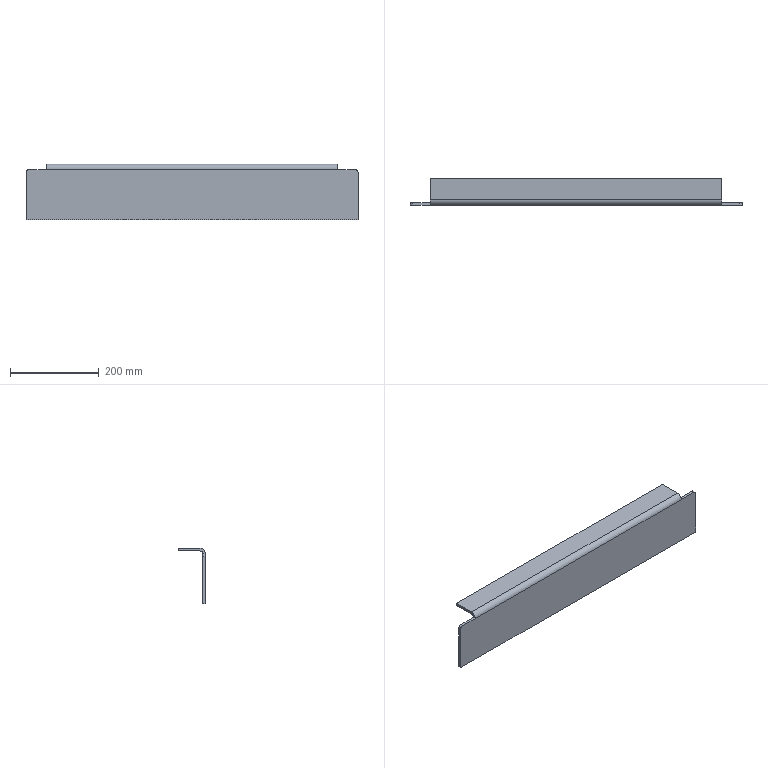Part | NX | features solid 2 | 1 solid | 16 faces | box 750 x 60 x 125 mm | volume 753725 mm3 | plane 12 | cylinder 4 | commonest cylinder face diameters 12 x3 24 x1
STEP:
#1=CARTESIAN_POINT('',(-345.,50.,-225.));
#2=VERTEX_POINT('',#1);
#3=CARTESIAN_POINT('',(-351.,50.,-219.));
#4=VERTEX_POINT('',#3);
#5=CARTESIAN_POINT('',(-351.,50.,-225.));
#6=DIRECTION('',(0.,-1.,0.));
#7=DIRECTION('',(-1.,0.,0.));
#8=AXIS2_PLACEMENT_3D('',#5,#6,#7);
#9=CIRCLE('',#8,6.);
#10=EDGE_CURVE('',#2,#4,#9,.T.);
#11=ORIENTED_EDGE('',*,*,#10,.F.);
#12=CARTESIAN_POINT('',(-345.,56.,-225.));
#13=VERTEX_POINT('',#12);
#14=CARTESIAN_POINT('',(-345.,48.,-225.));
#15=DIRECTION('',(0.,-1.,0.));
#16=VECTOR('',#15,1000.);
#17=LINE('',#14,#16);
#18=EDGE_CURVE('',#13,#2,#17,.T.);
#19=ORIENTED_EDGE('',*,*,#18,.F.);
#20=CARTESIAN_POINT('',(-351.,56.,-219.));
#21=VERTEX_POINT('',#20);
#22=CARTESIAN_POINT('',(-351.,56.,-225.));
#23=DIRECTION('',(0.,1.,0.));
#24=DIRECTION('',(-1.,0.,0.));
#25=AXIS2_PLACEMENT_3D('',#22,#23,#24);
#26=CIRCLE('',#25,6.);
#27=EDGE_CURVE('',#21,#13,#26,.T.);
#28=ORIENTED_EDGE('',*,*,#27,.F.);
#29=CARTESIAN_POINT('',(-351.,56.,-219.));
#30=DIRECTION('',(0.,1.,0.));
#31=VECTOR('',#30,1000.);
#32=LINE('',#29,#31);
#33=EDGE_CURVE('',#4,#21,#32,.T.);
#34=ORIENTED_EDGE('',*,*,#33,.F.);
#35=EDGE_LOOP('',(#11,#19,#28,#34));
#36=FACE_BOUND('',#35,.T.);
#37=CARTESIAN_POINT('',(-351.,56.,-225.));
#38=DIRECTION('',(0.,1.,0.));
#39=DIRECTION('',(-1.,0.,0.));
#40=AXIS2_PLACEMENT_3D('',#37,#38,#39);
#41=CYLINDRICAL_SURFACE('',#40,6.);
#42=ADVANCED_FACE('',(#36),#41,.T.);
#43=CARTESIAN_POINT('',(-1089.,50.,-219.));
#44=VERTEX_POINT('',#43);
#45=CARTESIAN_POINT('',(-1095.,50.,-225.));
#46=VERTEX_POINT('',#45);
#47=CARTESIAN_POINT('',(-1089.,50.,-225.));
#48=DIRECTION('',(0.,-1.,0.));
#49=DIRECTION('',(-1.,0.,0.));
#50=AXIS2_PLACEMENT_3D('',#47,#48,#49);
#51=CIRCLE('',#50,6.);
#52=EDGE_CURVE('',#44,#46,#51,.T.);
#53=ORIENTED_EDGE('',*,*,#52,.F.);
#54=CARTESIAN_POINT('',(-1089.,56.,-219.));
#55=VERTEX_POINT('',#54);
#56=CARTESIAN_POINT('',(-1089.,56.,-219.));
#57=DIRECTION('',(0.,-1.,0.));
#58=VECTOR('',#57,1000.);
#59=LINE('',#56,#58);
#60=EDGE_CURVE('',#55,#44,#59,.T.);
#61=ORIENTED_EDGE('',*,*,#60,.F.);
#62=CARTESIAN_POINT('',(-1095.,56.,-225.));
#63=VERTEX_POINT('',#62);
#64=CARTESIAN_POINT('',(-1089.,56.,-225.));
#65=DIRECTION('',(0.,1.,0.));
#66=DIRECTION('',(-1.,0.,0.));
#67=AXIS2_PLACEMENT_3D('',#64,#65,#66);
#68=CIRCLE('',#67,6.);
#69=EDGE_CURVE('',#63,#55,#68,.T.);
#70=ORIENTED_EDGE('',*,*,#69,.F.);
#71=CARTESIAN_POINT('',(-1095.,48.,-225.));
#72=DIRECTION('',(0.,1.,0.));
#73=VECTOR('',#72,1000.);
#74=LINE('',#71,#73);
#75=EDGE_CURVE('',#46,#63,#74,.T.);
#76=ORIENTED_EDGE('',*,*,#75,.F.);
#77=EDGE_LOOP('',(#53,#61,#70,#76));
#78=FACE_BOUND('',#77,.T.);
#79=CARTESIAN_POINT('',(-1089.,48.,-225.));
#80=DIRECTION('',(0.,1.,0.));
#81=DIRECTION('',(-1.,0.,0.));
#82=AXIS2_PLACEMENT_3D('',#79,#80,#81);
#83=CYLINDRICAL_SURFACE('',#82,6.);
#84=ADVANCED_FACE('',(#78),#83,.T.);
#85=CARTESIAN_POINT('',(-391.,62.,-213.));
#86=VERTEX_POINT('',#85);
#87=CARTESIAN_POINT('',(-391.,56.,-219.));
#88=VERTEX_POINT('',#87);
#89=CARTESIAN_POINT('',(-391.,62.,-219.));
#90=DIRECTION('',(1.,0.,0.));
#91=DIRECTION('',(0.,-1.,0.));
#92=AXIS2_PLACEMENT_3D('',#89,#90,#91);
#93=CIRCLE('',#92,6.);
#94=EDGE_CURVE('',#86,#88,#93,.T.);
#95=ORIENTED_EDGE('',*,*,#94,.T.);
#96=CARTESIAN_POINT('',(-1049.,56.,-219.));
#97=VERTEX_POINT('',#96);
#98=CARTESIAN_POINT('',(-1095.,56.,-219.));
#99=DIRECTION('',(-1.,0.,0.));
#100=VECTOR('',#99,1000.);
#101=LINE('',#98,#100);
#102=EDGE_CURVE('',#88,#97,#101,.T.);
#103=ORIENTED_EDGE('',*,*,#102,.T.);
#104=CARTESIAN_POINT('',(-1049.,62.,-213.));
#105=VERTEX_POINT('',#104);
#106=CARTESIAN_POINT('',(-1049.,62.,-219.));
#107=DIRECTION('',(-1.,0.,0.));
#108=DIRECTION('',(0.,-1.,0.));
#109=AXIS2_PLACEMENT_3D('',#106,#107,#108);
#110=CIRCLE('',#109,6.);
#111=EDGE_CURVE('',#97,#105,#110,.T.);
#112=ORIENTED_EDGE('',*,*,#111,.T.);
#113=CARTESIAN_POINT('',(-1049.,62.,-213.));
#114=DIRECTION('',(1.,0.,0.));
#115=VECTOR('',#114,1000.);
#116=LINE('',#113,#115);
#117=EDGE_CURVE('',#105,#86,#116,.T.);
#118=ORIENTED_EDGE('',*,*,#117,.T.);
#119=EDGE_LOOP('',(#95,#103,#112,#118));
#120=FACE_BOUND('',#119,.T.);
#121=CARTESIAN_POINT('',(-1095.,62.,-219.));
#122=DIRECTION('',(1.,0.,0.));
#123=DIRECTION('',(0.,1.,0.));
#124=AXIS2_PLACEMENT_3D('',#121,#122,#123);
#125=CYLINDRICAL_SURFACE('',#124,6.);
#126=ADVANCED_FACE('',(#120),#125,.F.);
#127=CARTESIAN_POINT('',(-391.,62.,-207.));
#128=VERTEX_POINT('',#127);
#129=CARTESIAN_POINT('',(-391.,50.,-219.));
#130=VERTEX_POINT('',#129);
#131=CARTESIAN_POINT('',(-391.,62.,-219.));
#132=DIRECTION('',(1.,0.,0.));
#133=DIRECTION('',(0.,1.,0.));
#134=AXIS2_PLACEMENT_3D('',#131,#132,#133);
#135=CIRCLE('',#134,12.);
#136=EDGE_CURVE('',#128,#130,#135,.T.);
#137=ORIENTED_EDGE('',*,*,#136,.F.);
#138=CARTESIAN_POINT('',(-1049.,62.,-207.));
#139=VERTEX_POINT('',#138);
#140=CARTESIAN_POINT('',(-1049.,62.,-207.));
#141=DIRECTION('',(1.,0.,0.));
#142=VECTOR('',#141,1000.);
#143=LINE('',#140,#142);
#144=EDGE_CURVE('',#139,#128,#143,.T.);
#145=ORIENTED_EDGE('',*,*,#144,.F.);
#146=CARTESIAN_POINT('',(-1049.,50.,-219.));
#147=VERTEX_POINT('',#146);
#148=CARTESIAN_POINT('',(-1049.,62.,-219.));
#149=DIRECTION('',(-1.,0.,0.));
#150=DIRECTION('',(0.,1.,0.));
#151=AXIS2_PLACEMENT_3D('',#148,#149,#150);
#152=CIRCLE('',#151,12.);
#153=EDGE_CURVE('',#147,#139,#152,.T.);
#154=ORIENTED_EDGE('',*,*,#153,.F.);
#155=CARTESIAN_POINT('',(-391.,50.,-219.));
#156=DIRECTION('',(-1.,0.,0.));
#157=VECTOR('',#156,1000.);
#158=LINE('',#155,#157);
#159=EDGE_CURVE('',#130,#147,#158,.T.);
#160=ORIENTED_EDGE('',*,*,#159,.F.);
#161=EDGE_LOOP('',(#137,#145,#154,#160));
#162=FACE_BOUND('',#161,.T.);
#163=CARTESIAN_POINT('',(-1095.,62.,-219.));
#164=DIRECTION('',(1.,0.,0.));
#165=DIRECTION('',(0.,1.,0.));
#166=AXIS2_PLACEMENT_3D('',#163,#164,#165);
#167=CYLINDRICAL_SURFACE('',#166,12.);
#168=ADVANCED_FACE('',(#162),#167,.T.);
#169=CARTESIAN_POINT('',(-391.,110.,-213.));
#170=VERTEX_POINT('',#169);
#171=CARTESIAN_POINT('',(-1049.,110.,-213.));
#172=VERTEX_POINT('',#171);
#173=CARTESIAN_POINT('',(-391.,110.,-213.));
#174=DIRECTION('',(-1.,0.,0.));
#175=VECTOR('',#174,1000.);
#176=LINE('',#173,#175);
#177=EDGE_CURVE('',#170,#172,#176,.T.);
#178=ORIENTED_EDGE('',*,*,#177,.T.);
#179=CARTESIAN_POINT('',(-1049.,110.,-207.));
#180=VERTEX_POINT('',#179);
#181=CARTESIAN_POINT('',(-1049.,110.,-207.));
#182=DIRECTION('',(0.,0.,-1.));
#183=VECTOR('',#182,1000.);
#184=LINE('',#181,#183);
#185=EDGE_CURVE('',#180,#172,#184,.T.);
#186=ORIENTED_EDGE('',*,*,#185,.F.);
#187=CARTESIAN_POINT('',(-391.,110.,-207.));
#188=VERTEX_POINT('',#187);
#189=CARTESIAN_POINT('',(-391.,110.,-207.));
#190=DIRECTION('',(-1.,0.,0.));
#191=VECTOR('',#190,1000.);
#192=LINE('',#189,#191);
#193=EDGE_CURVE('',#188,#180,#192,.T.);
#194=ORIENTED_EDGE('',*,*,#193,.F.);
#195=CARTESIAN_POINT('',(-391.,110.,-207.));
#196=DIRECTION('',(0.,0.,-1.));
#197=VECTOR('',#196,1000.);
#198=LINE('',#195,#197);
#199=EDGE_CURVE('',#188,#170,#198,.T.);
#200=ORIENTED_EDGE('',*,*,#199,.T.);
#201=EDGE_LOOP('',(#178,#186,#194,#200));
#202=FACE_BOUND('',#201,.T.);
#203=CARTESIAN_POINT('',(-391.,110.,-207.));
#204=DIRECTION('',(0.,-1.,0.));
#205=DIRECTION('',(-1.,0.,0.));
#206=AXIS2_PLACEMENT_3D('',#203,#204,#205);
#207=PLANE('',#206);
#208=ADVANCED_FACE('',(#202),#207,.F.);
#209=ORIENTED_EDGE('',*,*,#117,.F.);
#210=CARTESIAN_POINT('',(-1049.,54.931,-213.));
#211=DIRECTION('',(0.,-1.,0.));
#212=VECTOR('',#211,1000.);
#213=LINE('',#210,#212);
#214=EDGE_CURVE('',#172,#105,#213,.T.);
#215=ORIENTED_EDGE('',*,*,#214,.F.);
#216=ORIENTED_EDGE('',*,*,#177,.F.);
#217=CARTESIAN_POINT('',(-391.,54.931,-213.));
#218=DIRECTION('',(0.,1.,0.));
#219=VECTOR('',#218,1000.);
#220=LINE('',#217,#219);
#221=EDGE_CURVE('',#86,#170,#220,.T.);
#222=ORIENTED_EDGE('',*,*,#221,.F.);
#223=EDGE_LOOP('',(#209,#215,#216,#222));
#224=FACE_BOUND('',#223,.T.);
#225=CARTESIAN_POINT('',(-419.566,48.,-213.));
#226=DIRECTION('',(0.,0.,1.));
#227=DIRECTION('',(0.,-1.,0.));
#228=AXIS2_PLACEMENT_3D('',#225,#226,#227);
#229=PLANE('',#228);
#230=ADVANCED_FACE('',(#224),#229,.F.);
#231=CARTESIAN_POINT('',(-1049.,54.931,-207.));
#232=DIRECTION('',(0.,-1.,0.));
#233=VECTOR('',#232,1000.);
#234=LINE('',#231,#233);
#235=EDGE_CURVE('',#180,#139,#234,.T.);
#236=ORIENTED_EDGE('',*,*,#235,.T.);
#237=ORIENTED_EDGE('',*,*,#144,.T.);
#238=CARTESIAN_POINT('',(-391.,54.931,-207.));
#239=DIRECTION('',(0.,1.,0.));
#240=VECTOR('',#239,1000.);
#241=LINE('',#238,#240);
#242=EDGE_CURVE('',#128,#188,#241,.T.);
#243=ORIENTED_EDGE('',*,*,#242,.T.);
#244=ORIENTED_EDGE('',*,*,#193,.T.);
#245=EDGE_LOOP('',(#236,#237,#243,#244));
#246=FACE_BOUND('',#245,.T.);
#247=CARTESIAN_POINT('',(-419.566,48.,-207.));
#248=DIRECTION('',(0.,0.,1.));
#249=DIRECTION('',(0.,-1.,0.));
#250=AXIS2_PLACEMENT_3D('',#247,#248,#249);
#251=PLANE('',#250);
#252=ADVANCED_FACE('',(#246),#251,.T.);
#253=ORIENTED_EDGE('',*,*,#214,.T.);
#254=ORIENTED_EDGE('',*,*,#111,.F.);
#255=CARTESIAN_POINT('',(-1049.,50.,-219.));
#256=DIRECTION('',(0.,-1.,0.));
#257=VECTOR('',#256,1000.);
#258=LINE('',#255,#257);
#259=EDGE_CURVE('',#97,#147,#258,.T.);
#260=ORIENTED_EDGE('',*,*,#259,.T.);
#261=ORIENTED_EDGE('',*,*,#153,.T.);
#262=ORIENTED_EDGE('',*,*,#235,.F.);
#263=ORIENTED_EDGE('',*,*,#185,.T.);
#264=EDGE_LOOP('',(#253,#254,#260,#261,#262,#263));
#265=FACE_BOUND('',#264,.T.);
#266=CARTESIAN_POINT('',(-1049.,54.931,-207.));
#267=DIRECTION('',(1.,0.,0.));
#268=DIRECTION('',(0.,1.,0.));
#269=AXIS2_PLACEMENT_3D('',#266,#267,#268);
#270=PLANE('',#269);
#271=ADVANCED_FACE('',(#265),#270,.F.);
#272=ORIENTED_EDGE('',*,*,#242,.F.);
#273=ORIENTED_EDGE('',*,*,#136,.T.);
#274=CARTESIAN_POINT('',(-391.,50.,-219.));
#275=DIRECTION('',(0.,-1.,0.));
#276=VECTOR('',#275,1000.);
#277=LINE('',#274,#276);
#278=EDGE_CURVE('',#88,#130,#277,.T.);
#279=ORIENTED_EDGE('',*,*,#278,.F.);
#280=ORIENTED_EDGE('',*,*,#94,.F.);
#281=ORIENTED_EDGE('',*,*,#221,.T.);
#282=ORIENTED_EDGE('',*,*,#199,.F.);
#283=EDGE_LOOP('',(#272,#273,#279,#280,#281,#282));
#284=FACE_BOUND('',#283,.T.);
#285=CARTESIAN_POINT('',(-391.,54.931,-207.));
#286=DIRECTION('',(-1.,0.,0.));
#287=DIRECTION('',(0.,0.,1.));
#288=AXIS2_PLACEMENT_3D('',#285,#286,#287);
#289=PLANE('',#288);
#290=ADVANCED_FACE('',(#284),#289,.F.);
#291=CARTESIAN_POINT('',(-1095.,50.,-332.));
#292=VERTEX_POINT('',#291);
#293=CARTESIAN_POINT('',(-1095.,50.,-332.));
#294=DIRECTION('',(0.,0.,1.));
#295=VECTOR('',#294,1000.);
#296=LINE('',#293,#295);
#297=EDGE_CURVE('',#292,#46,#296,.T.);
#298=ORIENTED_EDGE('',*,*,#297,.T.);
#299=ORIENTED_EDGE('',*,*,#75,.T.);
#300=CARTESIAN_POINT('',(-1095.,56.,-332.));
#301=VERTEX_POINT('',#300);
#302=CARTESIAN_POINT('',(-1095.,56.,-332.));
#303=DIRECTION('',(0.,0.,1.));
#304=VECTOR('',#303,1000.);
#305=LINE('',#302,#304);
#306=EDGE_CURVE('',#301,#63,#305,.T.);
#307=ORIENTED_EDGE('',*,*,#306,.F.);
#308=CARTESIAN_POINT('',(-1095.,48.,-332.));
#309=DIRECTION('',(0.,-1.,0.));
#310=VECTOR('',#309,1000.);
#311=LINE('',#308,#310);
#312=EDGE_CURVE('',#301,#292,#311,.T.);
#313=ORIENTED_EDGE('',*,*,#312,.T.);
#314=EDGE_LOOP('',(#298,#299,#307,#313));
#315=FACE_BOUND('',#314,.T.);
#316=CARTESIAN_POINT('',(-1095.,48.,-338.));
#317=DIRECTION('',(1.,0.,0.));
#318=DIRECTION('',(0.,-1.,0.));
#319=AXIS2_PLACEMENT_3D('',#316,#317,#318);
#320=PLANE('',#319);
#321=ADVANCED_FACE('',(#315),#320,.F.);
#322=CARTESIAN_POINT('',(-364.,50.,-219.));
#323=DIRECTION('',(1.,0.,0.));
#324=VECTOR('',#323,1000.);
#325=LINE('',#322,#324);
#326=EDGE_CURVE('',#130,#4,#325,.T.);
#327=ORIENTED_EDGE('',*,*,#326,.T.);
#328=ORIENTED_EDGE('',*,*,#33,.T.);
#329=CARTESIAN_POINT('',(-364.,56.,-219.));
#330=DIRECTION('',(1.,0.,0.));
#331=VECTOR('',#330,1000.);
#332=LINE('',#329,#331);
#333=EDGE_CURVE('',#88,#21,#332,.T.);
#334=ORIENTED_EDGE('',*,*,#333,.F.);
#335=ORIENTED_EDGE('',*,*,#278,.T.);
#336=EDGE_LOOP('',(#327,#328,#334,#335));
#337=FACE_BOUND('',#336,.T.);
#338=CARTESIAN_POINT('',(-364.,56.,-219.));
#339=DIRECTION('',(0.,0.,-1.));
#340=DIRECTION('',(-1.,0.,0.));
#341=AXIS2_PLACEMENT_3D('',#338,#339,#340);
#342=PLANE('',#341);
#343=ADVANCED_FACE('',(#337),#342,.F.);
#344=ORIENTED_EDGE('',*,*,#306,.T.);
#345=ORIENTED_EDGE('',*,*,#69,.T.);
#346=CARTESIAN_POINT('',(-364.,56.,-219.));
#347=DIRECTION('',(1.,0.,0.));
#348=VECTOR('',#347,1000.);
#349=LINE('',#346,#348);
#350=EDGE_CURVE('',#55,#97,#349,.T.);
#351=ORIENTED_EDGE('',*,*,#350,.T.);
#352=ORIENTED_EDGE('',*,*,#102,.F.);
#353=ORIENTED_EDGE('',*,*,#333,.T.);
#354=ORIENTED_EDGE('',*,*,#27,.T.);
#355=CARTESIAN_POINT('',(-345.,56.,-332.));
#356=VERTEX_POINT('',#355);
#357=CARTESIAN_POINT('',(-345.,56.,-332.));
#358=DIRECTION('',(0.,0.,-1.));
#359=VECTOR('',#358,1000.);
#360=LINE('',#357,#359);
#361=EDGE_CURVE('',#13,#356,#360,.T.);
#362=ORIENTED_EDGE('',*,*,#361,.T.);
#363=CARTESIAN_POINT('',(-364.,56.,-332.));
#364=DIRECTION('',(-1.,0.,0.));
#365=VECTOR('',#364,1000.);
#366=LINE('',#363,#365);
#367=EDGE_CURVE('',#356,#301,#366,.T.);
#368=ORIENTED_EDGE('',*,*,#367,.T.);
#369=EDGE_LOOP('',(#344,#345,#351,#352,#353,#354,#362,#368));
#370=FACE_BOUND('',#369,.T.);
#371=CARTESIAN_POINT('',(-364.,56.,-332.));
#372=DIRECTION('',(0.,1.,0.));
#373=DIRECTION('',(1.,0.,0.));
#374=AXIS2_PLACEMENT_3D('',#371,#372,#373);
#375=PLANE('',#374);
#376=ADVANCED_FACE('',(#370),#375,.T.);
#377=ORIENTED_EDGE('',*,*,#312,.F.);
#378=ORIENTED_EDGE('',*,*,#367,.F.);
#379=CARTESIAN_POINT('',(-345.,50.,-332.));
#380=VERTEX_POINT('',#379);
#381=CARTESIAN_POINT('',(-345.,48.,-332.));
#382=DIRECTION('',(0.,-1.,0.));
#383=VECTOR('',#382,1000.);
#384=LINE('',#381,#383);
#385=EDGE_CURVE('',#356,#380,#384,.T.);
#386=ORIENTED_EDGE('',*,*,#385,.T.);
#387=CARTESIAN_POINT('',(-364.,50.,-332.));
#388=DIRECTION('',(-1.,0.,0.));
#389=VECTOR('',#388,1000.);
#390=LINE('',#387,#389);
#391=EDGE_CURVE('',#380,#292,#390,.T.);
#392=ORIENTED_EDGE('',*,*,#391,.T.);
#393=EDGE_LOOP('',(#377,#378,#386,#392));
#394=FACE_BOUND('',#393,.T.);
#395=CARTESIAN_POINT('',(-364.,48.,-332.));
#396=DIRECTION('',(0.,0.,1.));
#397=DIRECTION('',(0.,-1.,0.));
#398=AXIS2_PLACEMENT_3D('',#395,#396,#397);
#399=PLANE('',#398);
#400=ADVANCED_FACE('',(#394),#399,.F.);
#401=CARTESIAN_POINT('',(-364.,50.,-219.));
#402=DIRECTION('',(1.,0.,0.));
#403=VECTOR('',#402,1000.);
#404=LINE('',#401,#403);
#405=EDGE_CURVE('',#44,#147,#404,.T.);
#406=ORIENTED_EDGE('',*,*,#405,.F.);
#407=ORIENTED_EDGE('',*,*,#52,.T.);
#408=ORIENTED_EDGE('',*,*,#297,.F.);
#409=ORIENTED_EDGE('',*,*,#391,.F.);
#410=CARTESIAN_POINT('',(-345.,50.,-332.));
#411=DIRECTION('',(0.,0.,1.));
#412=VECTOR('',#411,1000.);
#413=LINE('',#410,#412);
#414=EDGE_CURVE('',#380,#2,#413,.T.);
#415=ORIENTED_EDGE('',*,*,#414,.T.);
#416=ORIENTED_EDGE('',*,*,#10,.T.);
#417=ORIENTED_EDGE('',*,*,#326,.F.);
#418=ORIENTED_EDGE('',*,*,#159,.T.);
#419=EDGE_LOOP('',(#406,#407,#408,#409,#415,#416,#417,#418));
#420=FACE_BOUND('',#419,.T.);
#421=CARTESIAN_POINT('',(-364.,50.,-332.));
#422=DIRECTION('',(0.,1.,0.));
#423=DIRECTION('',(1.,0.,0.));
#424=AXIS2_PLACEMENT_3D('',#421,#422,#423);
#425=PLANE('',#424);
#426=ADVANCED_FACE('',(#420),#425,.F.);
#427=ORIENTED_EDGE('',*,*,#361,.F.);
#428=ORIENTED_EDGE('',*,*,#18,.T.);
#429=ORIENTED_EDGE('',*,*,#414,.F.);
#430=ORIENTED_EDGE('',*,*,#385,.F.);
#431=EDGE_LOOP('',(#427,#428,#429,#430));
#432=FACE_BOUND('',#431,.T.);
#433=CARTESIAN_POINT('',(-345.,48.,-338.));
#434=DIRECTION('',(-1.,0.,0.));
#435=DIRECTION('',(0.,0.,1.));
#436=AXIS2_PLACEMENT_3D('',#433,#434,#435);
#437=PLANE('',#436);
#438=ADVANCED_FACE('',(#432),#437,.F.);
#439=ORIENTED_EDGE('',*,*,#350,.F.);
#440=ORIENTED_EDGE('',*,*,#60,.T.);
#441=ORIENTED_EDGE('',*,*,#405,.T.);
#442=ORIENTED_EDGE('',*,*,#259,.F.);
#443=EDGE_LOOP('',(#439,#440,#441,#442));
#444=FACE_BOUND('',#443,.T.);
#445=CARTESIAN_POINT('',(-364.,56.,-219.));
#446=DIRECTION('',(0.,0.,-1.));
#447=DIRECTION('',(-1.,0.,0.));
#448=AXIS2_PLACEMENT_3D('',#445,#446,#447);
#449=PLANE('',#448);
#450=ADVANCED_FACE('',(#444),#449,.F.);
#451=CLOSED_SHELL('',(#42,#84,#126,#168,#208,#230,#252,#271,#290,#321,#343,#376,#400,#426,#438,#450));
#452=MANIFOLD_SOLID_BREP('',#451);
#453=(LENGTH_UNIT()NAMED_UNIT(*)SI_UNIT(.MILLI.,.METRE.));
#454=UNCERTAINTY_MEASURE_WITH_UNIT(LENGTH_MEASURE(0.00001),#453,'','');
#455=(NAMED_UNIT(*)PLANE_ANGLE_UNIT()SI_UNIT($,.RADIAN.));
#456=(NAMED_UNIT(*)SI_UNIT($,.STERADIAN.)SOLID_ANGLE_UNIT());
#457=(GEOMETRIC_REPRESENTATION_CONTEXT(3)GLOBAL_UNCERTAINTY_ASSIGNED_CONTEXT((#454))GLOBAL_UNIT_ASSIGNED_CONTEXT((#453,#455,#456))REPRESENTATION_CONTEXT('',''));
#458=ADVANCED_BREP_SHAPE_REPRESENTATION('',(#452),#457);